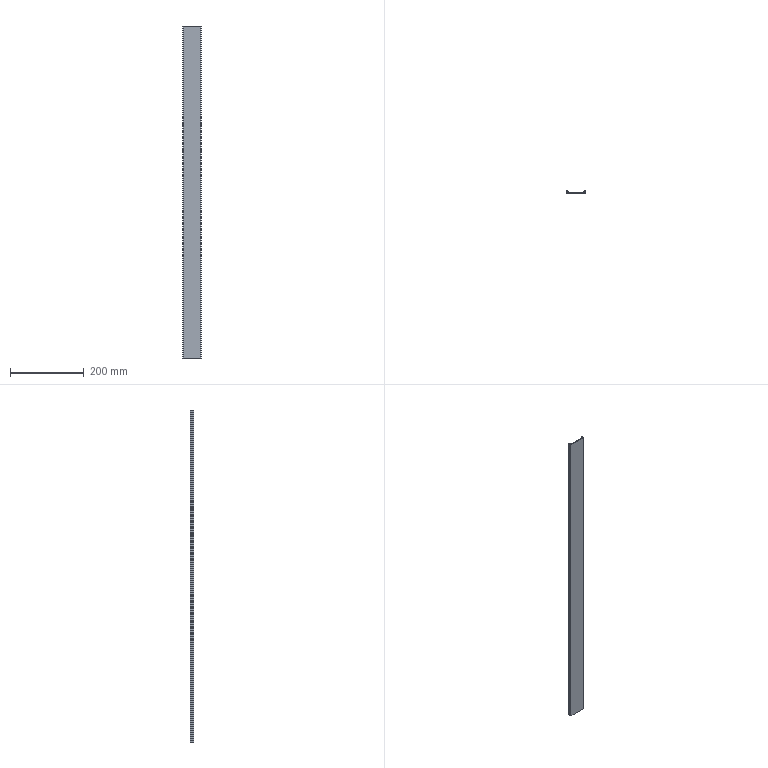Part | STEP file | 31E-01001CC13 | 1 solid | 32 faces | box 50 x 9.195 x 900 mm | volume 78943 mm3 | cylinder 16 | plane 16 | commonest cylinder face diameters 1 x8 1.2 x6 2 x2
STEP:
#1=CARTESIAN_POINT('',(0.2485,8.595,450.));
#2=VERTEX_POINT('',#1);
#3=CARTESIAN_POINT('',(0.4243,8.171,450.));
#4=VERTEX_POINT('',#3);
#5=CARTESIAN_POINT('',(0.8485,8.595,450.));
#6=DIRECTION('',(0.,0.,-1.));
#7=AXIS2_PLACEMENT_3D('',#5,#6,$);
#8=CIRCLE('',#7,0.6);
#9=EDGE_CURVE('',#2,#4,#8,.F.);
#10=ORIENTED_EDGE('',*,*,#9,.F.);
#11=CARTESIAN_POINT('',(0.2485,8.595,-450.));
#12=VERTEX_POINT('',#11);
#13=CARTESIAN_POINT('',(0.2485,8.595,450.));
#14=DIRECTION('',(0.,0.,-1.));
#15=VECTOR('',#14,1.);
#16=LINE('',#13,#15);
#17=EDGE_CURVE('',#2,#12,#16,.T.);
#18=ORIENTED_EDGE('',*,*,#17,.T.);
#19=CARTESIAN_POINT('',(0.4243,8.171,-450.));
#20=VERTEX_POINT('',#19);
#21=CARTESIAN_POINT('',(0.8485,8.595,-450.));
#22=DIRECTION('',(0.,0.,-1.));
#23=AXIS2_PLACEMENT_3D('',#21,#22,$);
#24=CIRCLE('',#23,0.6);
#25=EDGE_CURVE('',#20,#12,#24,.T.);
#26=ORIENTED_EDGE('',*,*,#25,.F.);
#27=CARTESIAN_POINT('',(0.4243,8.171,450.));
#28=DIRECTION('',(0.,0.,-1.));
#29=VECTOR('',#28,1.);
#30=LINE('',#27,#29);
#31=EDGE_CURVE('',#4,#20,#30,.T.);
#32=ORIENTED_EDGE('',*,*,#31,.F.);
#33=EDGE_LOOP('',(#10,#18,#26,#32));
#34=FACE_OUTER_BOUND('',#33,.T.);
#35=CARTESIAN_POINT('',(0.8485,8.595,450.));
#36=DIRECTION('',(0.,0.,-1.));
#37=DIRECTION('',(1.,0.,0.));
#38=AXIS2_PLACEMENT_3D('',#35,#36,#37);
#39=CYLINDRICAL_SURFACE('',#38,0.6);
#40=ADVANCED_FACE('',(#34),#39,.T.);
#41=CARTESIAN_POINT('',(1.273,9.019,450.));
#42=VERTEX_POINT('',#41);
#43=CARTESIAN_POINT('',(0.4243,9.019,450.));
#44=VERTEX_POINT('',#43);
#45=CARTESIAN_POINT('',(1.273,9.019,450.));
#46=CARTESIAN_POINT('',(1.219,9.073,450.));
#47=CARTESIAN_POINT('',(1.158,9.118,450.));
#48=CARTESIAN_POINT('',(1.089,9.152,450.));
#49=CARTESIAN_POINT('',(0.9442,9.199,450.));
#50=CARTESIAN_POINT('',(0.7916,9.2,450.));
#51=CARTESIAN_POINT('',(0.7159,9.188,450.));
#52=CARTESIAN_POINT('',(0.6071,9.152,450.));
#53=CARTESIAN_POINT('',(0.5104,9.093,450.));
#54=CARTESIAN_POINT('',(0.4796,9.07,450.));
#55=CARTESIAN_POINT('',(0.4509,9.046,450.));
#56=CARTESIAN_POINT('',(0.4243,9.019,450.));
#57=B_SPLINE_CURVE_WITH_KNOTS('',5,(#45,#46,#47,#48,#49,#50,#51,#52,#53,#54,#55,#56),.UNSPECIFIED.,.F.,.U.,(6,3,3,6),(0.,0.5331,1.066,1.332),.UNSPECIFIED.);
#58=EDGE_CURVE('',#42,#44,#57,.T.);
#59=ORIENTED_EDGE('',*,*,#58,.T.);
#60=CARTESIAN_POINT('',(0.4243,9.019,450.));
#61=CARTESIAN_POINT('',(0.3843,8.979,450.));
#62=CARTESIAN_POINT('',(0.349,8.935,450.));
#63=CARTESIAN_POINT('',(0.3192,8.886,450.));
#64=CARTESIAN_POINT('',(0.2795,8.8,450.));
#65=CARTESIAN_POINT('',(0.2574,8.708,450.));
#66=CARTESIAN_POINT('',(0.2515,8.67,450.));
#67=CARTESIAN_POINT('',(0.2485,8.633,450.));
#68=CARTESIAN_POINT('',(0.2485,8.595,450.));
#69=B_SPLINE_CURVE_WITH_KNOTS('',5,(#60,#61,#62,#63,#64,#65,#66,#67,#68),.UNSPECIFIED.,.F.,.U.,(6,3,6),(0.,0.3999,0.6659),.UNSPECIFIED.);
#70=EDGE_CURVE('',#44,#2,#69,.T.);
#71=ORIENTED_EDGE('',*,*,#70,.T.);
#72=ORIENTED_EDGE('',*,*,#9,.T.);
#73=CARTESIAN_POINT('',(2.898,5.697,450.));
#74=VERTEX_POINT('',#73);
#75=CARTESIAN_POINT('',(1.661,6.934,450.));
#76=DIRECTION('',(0.7071,-0.7071,0.));
#77=VECTOR('',#76,1.);
#78=LINE('',#75,#77);
#79=EDGE_CURVE('',#4,#74,#78,.T.);
#80=ORIENTED_EDGE('',*,*,#79,.T.);
#81=CARTESIAN_POINT('',(0.3706,5.02,450.));
#82=VERTEX_POINT('',#81);
#83=CARTESIAN_POINT('',(1.634,5.359,450.));
#84=DIRECTION('',(-0.9659,-0.2588,0.));
#85=VECTOR('',#84,1.);
#86=LINE('',#83,#85);
#87=EDGE_CURVE('',#74,#82,#86,.T.);
#88=ORIENTED_EDGE('',*,*,#87,.T.);
#89=CARTESIAN_POINT('',(0.,4.537,450.));
#90=VERTEX_POINT('',#89);
#91=CARTESIAN_POINT('',(0.3706,5.02,450.));
#92=CARTESIAN_POINT('',(0.32,5.007,450.));
#93=CARTESIAN_POINT('',(0.2712,4.986,450.));
#94=CARTESIAN_POINT('',(0.2253,4.96,450.));
#95=CARTESIAN_POINT('',(0.1416,4.896,450.));
#96=CARTESIAN_POINT('',(0.07725,4.812,450.));
#97=CARTESIAN_POINT('',(0.05076,4.766,450.));
#98=CARTESIAN_POINT('',(0.02052,4.693,450.));
#99=CARTESIAN_POINT('',(0.005155,4.616,450.));
#100=CARTESIAN_POINT('',(0.001709,4.589,450.));
#101=CARTESIAN_POINT('',(0.,4.563,450.));
#102=CARTESIAN_POINT('',(0.,4.537,450.));
#103=B_SPLINE_CURVE_WITH_KNOTS('',5,(#91,#92,#93,#94,#95,#96,#97,#98,#99,#100,#101,#102),.UNSPECIFIED.,.F.,.U.,(6,3,3,6),(0.,0.3702,0.7405,0.9253),.UNSPECIFIED.);
#104=EDGE_CURVE('',#82,#90,#103,.T.);
#105=ORIENTED_EDGE('',*,*,#104,.T.);
#106=CARTESIAN_POINT('',(0.,1.,450.));
#107=VERTEX_POINT('',#106);
#108=CARTESIAN_POINT('',(0.,2.769,450.));
#109=DIRECTION('',(0.,-1.,0.));
#110=VECTOR('',#109,1.);
#111=LINE('',#108,#110);
#112=EDGE_CURVE('',#90,#107,#111,.T.);
#113=ORIENTED_EDGE('',*,*,#112,.T.);
#114=CARTESIAN_POINT('',(1.,0.,450.));
#115=VERTEX_POINT('',#114);
#116=CARTESIAN_POINT('',(0.,1.,450.));
#117=CARTESIAN_POINT('',(0.,0.902,450.));
#118=CARTESIAN_POINT('',(0.012,0.804,450.));
#119=CARTESIAN_POINT('',(0.036,0.708,450.));
#120=CARTESIAN_POINT('',(0.107,0.5238,450.));
#121=CARTESIAN_POINT('',(0.2204,0.3622,450.));
#122=CARTESIAN_POINT('',(0.2868,0.2888,450.));
#123=CARTESIAN_POINT('',(0.4361,0.1597,450.));
#124=CARTESIAN_POINT('',(0.6122,0.0704,450.));
#125=CARTESIAN_POINT('',(0.7053,0.03682,450.));
#126=CARTESIAN_POINT('',(0.8215,0.01049,450.));
#127=CARTESIAN_POINT('',(0.9393,0.001534,450.));
#128=CARTESIAN_POINT('',(0.9596,0.0005109,450.));
#129=CARTESIAN_POINT('',(0.9798,0.000000001,450.));
#130=CARTESIAN_POINT('',(1.,0.000000001,450.));
#131=B_SPLINE_CURVE_WITH_KNOTS('',5,(#116,#117,#118,#119,#120,#121,#122,#123,#124,#125,#126,#127,#128,#129,#130),.UNSPECIFIED.,.F.,.U.,(6,3,3,3,6),(0.,0.6928,1.386,2.078,2.221),.UNSPECIFIED.);
#132=EDGE_CURVE('',#107,#115,#131,.T.);
#133=ORIENTED_EDGE('',*,*,#132,.T.);
#134=CARTESIAN_POINT('',(49.,0.,450.));
#135=VERTEX_POINT('',#134);
#136=CARTESIAN_POINT('',(25.,0.000000001,450.));
#137=DIRECTION('',(1.,0.,0.));
#138=VECTOR('',#137,1.);
#139=LINE('',#136,#138);
#140=EDGE_CURVE('',#115,#135,#139,.T.);
#141=ORIENTED_EDGE('',*,*,#140,.T.);
#142=CARTESIAN_POINT('',(50.,1.,450.));
#143=VERTEX_POINT('',#142);
#144=CARTESIAN_POINT('',(49.,0.000000001,450.));
#145=CARTESIAN_POINT('',(49.098,0.000000001,450.));
#146=CARTESIAN_POINT('',(49.196,0.012,450.));
#147=CARTESIAN_POINT('',(49.292,0.036,450.));
#148=CARTESIAN_POINT('',(49.476,0.107,450.));
#149=CARTESIAN_POINT('',(49.638,0.2204,450.));
#150=CARTESIAN_POINT('',(49.711,0.2868,450.));
#151=CARTESIAN_POINT('',(49.84,0.4361,450.));
#152=CARTESIAN_POINT('',(49.93,0.6122,450.));
#153=CARTESIAN_POINT('',(49.963,0.7053,450.));
#154=CARTESIAN_POINT('',(49.99,0.8215,450.));
#155=CARTESIAN_POINT('',(49.998,0.9393,450.));
#156=CARTESIAN_POINT('',(49.999,0.9596,450.));
#157=CARTESIAN_POINT('',(50.,0.9798,450.));
#158=CARTESIAN_POINT('',(50.,1.,450.));
#159=B_SPLINE_CURVE_WITH_KNOTS('',5,(#144,#145,#146,#147,#148,#149,#150,#151,#152,#153,#154,#155,#156,#157,#158),.UNSPECIFIED.,.F.,.U.,(6,3,3,3,6),(0.,0.6928,1.386,2.078,2.221),.UNSPECIFIED.);
#160=EDGE_CURVE('',#135,#143,#159,.T.);
#161=ORIENTED_EDGE('',*,*,#160,.T.);
#162=CARTESIAN_POINT('',(50.,4.537,450.));
#163=VERTEX_POINT('',#162);
#164=CARTESIAN_POINT('',(50.,2.769,450.));
#165=DIRECTION('',(0.,1.,0.));
#166=VECTOR('',#165,1.);
#167=LINE('',#164,#166);
#168=EDGE_CURVE('',#143,#163,#167,.T.);
#169=ORIENTED_EDGE('',*,*,#168,.T.);
#170=CARTESIAN_POINT('',(49.629,5.02,450.));
#171=VERTEX_POINT('',#170);
#172=CARTESIAN_POINT('',(50.,4.537,450.));
#173=CARTESIAN_POINT('',(50.,4.589,450.));
#174=CARTESIAN_POINT('',(49.993,4.642,450.));
#175=CARTESIAN_POINT('',(49.979,4.693,450.));
#176=CARTESIAN_POINT('',(49.939,4.791,450.));
#177=CARTESIAN_POINT('',(49.875,4.874,450.));
#178=CARTESIAN_POINT('',(49.837,4.912,450.));
#179=CARTESIAN_POINT('',(49.774,4.96,450.));
#180=CARTESIAN_POINT('',(49.704,4.995,450.));
#181=CARTESIAN_POINT('',(49.679,5.005,450.));
#182=CARTESIAN_POINT('',(49.655,5.013,450.));
#183=CARTESIAN_POINT('',(49.629,5.02,450.));
#184=B_SPLINE_CURVE_WITH_KNOTS('',5,(#172,#173,#174,#175,#176,#177,#178,#179,#180,#181,#182,#183),.UNSPECIFIED.,.F.,.U.,(6,3,3,6),(0.,0.3702,0.7405,0.9253),.UNSPECIFIED.);
#185=EDGE_CURVE('',#163,#171,#184,.T.);
#186=ORIENTED_EDGE('',*,*,#185,.T.);
#187=CARTESIAN_POINT('',(47.102,5.697,450.));
#188=VERTEX_POINT('',#187);
#189=CARTESIAN_POINT('',(48.366,5.359,450.));
#190=DIRECTION('',(-0.9659,0.2588,0.));
#191=VECTOR('',#190,1.);
#192=LINE('',#189,#191);
#193=EDGE_CURVE('',#171,#188,#192,.T.);
#194=ORIENTED_EDGE('',*,*,#193,.T.);
#195=CARTESIAN_POINT('',(49.576,8.171,450.));
#196=VERTEX_POINT('',#195);
#197=CARTESIAN_POINT('',(48.339,6.934,450.));
#198=DIRECTION('',(0.7071,0.7071,0.));
#199=VECTOR('',#198,1.);
#200=LINE('',#197,#199);
#201=EDGE_CURVE('',#188,#196,#200,.T.);
#202=ORIENTED_EDGE('',*,*,#201,.T.);
#203=CARTESIAN_POINT('',(49.751,8.595,450.));
#204=VERTEX_POINT('',#203);
#205=CARTESIAN_POINT('',(49.576,8.171,450.));
#206=CARTESIAN_POINT('',(49.629,8.224,450.));
#207=CARTESIAN_POINT('',(49.674,8.286,450.));
#208=CARTESIAN_POINT('',(49.709,8.354,450.));
#209=CARTESIAN_POINT('',(49.738,8.445,450.));
#210=CARTESIAN_POINT('',(49.749,8.539,450.));
#211=CARTESIAN_POINT('',(49.751,8.557,450.));
#212=CARTESIAN_POINT('',(49.751,8.576,450.));
#213=CARTESIAN_POINT('',(49.751,8.595,450.));
#214=B_SPLINE_CURVE_WITH_KNOTS('',5,(#205,#206,#207,#208,#209,#210,#211,#212,#213),.UNSPECIFIED.,.F.,.U.,(6,3,6),(0.,0.5331,0.6664),.UNSPECIFIED.);
#215=EDGE_CURVE('',#196,#204,#214,.T.);
#216=ORIENTED_EDGE('',*,*,#215,.T.);
#217=CARTESIAN_POINT('',(49.576,9.019,450.));
#218=VERTEX_POINT('',#217);
#219=CARTESIAN_POINT('',(49.751,8.595,450.));
#220=CARTESIAN_POINT('',(49.751,8.652,450.));
#221=CARTESIAN_POINT('',(49.745,8.708,450.));
#222=CARTESIAN_POINT('',(49.731,8.764,450.));
#223=CARTESIAN_POINT('',(49.699,8.853,450.));
#224=CARTESIAN_POINT('',(49.649,8.933,450.));
#225=CARTESIAN_POINT('',(49.627,8.964,450.));
#226=CARTESIAN_POINT('',(49.602,8.993,450.));
#227=CARTESIAN_POINT('',(49.576,9.019,450.));
#228=B_SPLINE_CURVE_WITH_KNOTS('',5,(#219,#220,#221,#222,#223,#224,#225,#226,#227),.UNSPECIFIED.,.F.,.U.,(6,3,6),(0.6664,1.066,1.332),.UNSPECIFIED.);
#229=EDGE_CURVE('',#204,#218,#228,.T.);
#230=ORIENTED_EDGE('',*,*,#229,.T.);
#231=CARTESIAN_POINT('',(48.727,9.019,450.));
#232=VERTEX_POINT('',#231);
#233=CARTESIAN_POINT('',(49.576,9.019,450.));
#234=CARTESIAN_POINT('',(49.522,9.073,450.));
#235=CARTESIAN_POINT('',(49.461,9.118,450.));
#236=CARTESIAN_POINT('',(49.392,9.152,450.));
#237=CARTESIAN_POINT('',(49.247,9.199,450.));
#238=CARTESIAN_POINT('',(49.095,9.2,450.));
#239=CARTESIAN_POINT('',(49.019,9.188,450.));
#240=CARTESIAN_POINT('',(48.91,9.152,450.));
#241=CARTESIAN_POINT('',(48.813,9.093,450.));
#242=CARTESIAN_POINT('',(48.782,9.07,450.));
#243=CARTESIAN_POINT('',(48.754,9.046,450.));
#244=CARTESIAN_POINT('',(48.727,9.019,450.));
#245=B_SPLINE_CURVE_WITH_KNOTS('',5,(#233,#234,#235,#236,#237,#238,#239,#240,#241,#242,#243,#244),.UNSPECIFIED.,.F.,.U.,(6,3,3,6),(0.,0.5331,1.066,1.332),.UNSPECIFIED.);
#246=EDGE_CURVE('',#218,#232,#245,.T.);
#247=ORIENTED_EDGE('',*,*,#246,.T.);
#248=CARTESIAN_POINT('',(45.396,5.688,450.));
#249=VERTEX_POINT('',#248);
#250=CARTESIAN_POINT('',(47.062,7.354,450.));
#251=DIRECTION('',(-0.7071,-0.7071,0.));
#252=VECTOR('',#251,1.);
#253=LINE('',#250,#252);
#254=EDGE_CURVE('',#232,#249,#253,.T.);
#255=ORIENTED_EDGE('',*,*,#254,.T.);
#256=CARTESIAN_POINT('',(45.25,5.335,450.));
#257=VERTEX_POINT('',#256);
#258=CARTESIAN_POINT('',(45.396,5.688,450.));
#259=CARTESIAN_POINT('',(45.363,5.655,450.));
#260=CARTESIAN_POINT('',(45.334,5.618,450.));
#261=CARTESIAN_POINT('',(45.309,5.577,450.));
#262=CARTESIAN_POINT('',(45.276,5.506,450.));
#263=CARTESIAN_POINT('',(45.257,5.429,450.));
#264=CARTESIAN_POINT('',(45.252,5.398,450.));
#265=CARTESIAN_POINT('',(45.25,5.366,450.));
#266=CARTESIAN_POINT('',(45.25,5.335,450.));
#267=B_SPLINE_CURVE_WITH_KNOTS('',5,(#258,#259,#260,#261,#262,#263,#264,#265,#266),.UNSPECIFIED.,.F.,.U.,(6,3,6),(0.,0.3332,0.5549),.UNSPECIFIED.);
#268=EDGE_CURVE('',#249,#257,#267,.T.);
#269=ORIENTED_EDGE('',*,*,#268,.T.);
#270=CARTESIAN_POINT('',(45.621,4.852,450.));
#271=VERTEX_POINT('',#270);
#272=CARTESIAN_POINT('',(45.25,5.335,450.));
#273=CARTESIAN_POINT('',(45.25,5.283,450.));
#274=CARTESIAN_POINT('',(45.257,5.23,450.));
#275=CARTESIAN_POINT('',(45.27,5.179,450.));
#276=CARTESIAN_POINT('',(45.311,5.081,450.));
#277=CARTESIAN_POINT('',(45.375,4.998,450.));
#278=CARTESIAN_POINT('',(45.413,4.96,450.));
#279=CARTESIAN_POINT('',(45.476,4.912,450.));
#280=CARTESIAN_POINT('',(45.546,4.877,450.));
#281=CARTESIAN_POINT('',(45.57,4.867,450.));
#282=CARTESIAN_POINT('',(45.595,4.859,450.));
#283=CARTESIAN_POINT('',(45.621,4.852,450.));
#284=B_SPLINE_CURVE_WITH_KNOTS('',5,(#272,#273,#274,#275,#276,#277,#278,#279,#280,#281,#282,#283),.UNSPECIFIED.,.F.,.U.,(6,3,3,6),(0.,0.3702,0.7405,0.9253),.UNSPECIFIED.);
#285=EDGE_CURVE('',#257,#271,#284,.T.);
#286=ORIENTED_EDGE('',*,*,#285,.T.);
#287=CARTESIAN_POINT('',(48.8,4.,450.));
#288=VERTEX_POINT('',#287);
#289=CARTESIAN_POINT('',(47.21,4.426,450.));
#290=DIRECTION('',(0.9659,-0.2588,0.));
#291=VECTOR('',#290,1.);
#292=LINE('',#289,#291);
#293=EDGE_CURVE('',#271,#288,#292,.T.);
#294=ORIENTED_EDGE('',*,*,#293,.T.);
#295=CARTESIAN_POINT('',(48.8,1.7,450.));
#296=VERTEX_POINT('',#295);
#297=CARTESIAN_POINT('',(48.8,2.85,450.));
#298=DIRECTION('',(0.,-1.,0.));
#299=VECTOR('',#298,1.);
#300=LINE('',#297,#299);
#301=EDGE_CURVE('',#288,#296,#300,.T.);
#302=ORIENTED_EDGE('',*,*,#301,.T.);
#303=CARTESIAN_POINT('',(48.3,1.2,450.));
#304=VERTEX_POINT('',#303);
#305=CARTESIAN_POINT('',(48.3,1.7,450.));
#306=DIRECTION('',(0.,0.,-1.));
#307=AXIS2_PLACEMENT_3D('',#305,#306,$);
#308=CIRCLE('',#307,0.5);
#309=EDGE_CURVE('',#296,#304,#308,.T.);
#310=ORIENTED_EDGE('',*,*,#309,.T.);
#311=CARTESIAN_POINT('',(1.7,1.2,450.));
#312=VERTEX_POINT('',#311);
#313=CARTESIAN_POINT('',(25.,1.2,450.));
#314=DIRECTION('',(-1.,0.,0.));
#315=VECTOR('',#314,1.);
#316=LINE('',#313,#315);
#317=EDGE_CURVE('',#304,#312,#316,.T.);
#318=ORIENTED_EDGE('',*,*,#317,.T.);
#319=CARTESIAN_POINT('',(1.2,1.7,450.));
#320=VERTEX_POINT('',#319);
#321=CARTESIAN_POINT('',(1.7,1.7,450.));
#322=DIRECTION('',(0.,0.,-1.));
#323=AXIS2_PLACEMENT_3D('',#321,#322,$);
#324=CIRCLE('',#323,0.5);
#325=EDGE_CURVE('',#312,#320,#324,.T.);
#326=ORIENTED_EDGE('',*,*,#325,.T.);
#327=CARTESIAN_POINT('',(1.2,4.,450.));
#328=VERTEX_POINT('',#327);
#329=CARTESIAN_POINT('',(1.2,2.85,450.));
#330=DIRECTION('',(0.,1.,0.));
#331=VECTOR('',#330,1.);
#332=LINE('',#329,#331);
#333=EDGE_CURVE('',#320,#328,#332,.T.);
#334=ORIENTED_EDGE('',*,*,#333,.T.);
#335=CARTESIAN_POINT('',(4.379,4.852,450.));
#336=VERTEX_POINT('',#335);
#337=CARTESIAN_POINT('',(2.79,4.426,450.));
#338=DIRECTION('',(0.9659,0.2588,0.));
#339=VECTOR('',#338,1.);
#340=LINE('',#337,#339);
#341=EDGE_CURVE('',#328,#336,#340,.T.);
#342=ORIENTED_EDGE('',*,*,#341,.T.);
#343=CARTESIAN_POINT('',(4.75,5.335,450.));
#344=VERTEX_POINT('',#343);
#345=CARTESIAN_POINT('',(4.379,4.852,450.));
#346=CARTESIAN_POINT('',(4.446,4.87,450.));
#347=CARTESIAN_POINT('',(4.51,4.899,450.));
#348=CARTESIAN_POINT('',(4.568,4.94,450.));
#349=CARTESIAN_POINT('',(4.662,5.034,450.));
#350=CARTESIAN_POINT('',(4.722,5.152,450.));
#351=CARTESIAN_POINT('',(4.741,5.212,450.));
#352=CARTESIAN_POINT('',(4.75,5.273,450.));
#353=CARTESIAN_POINT('',(4.75,5.335,450.));
#354=B_SPLINE_CURVE_WITH_KNOTS('',5,(#345,#346,#347,#348,#349,#350,#351,#352,#353),.UNSPECIFIED.,.F.,.U.,(6,3,6),(0.,0.4899,0.9256),.UNSPECIFIED.);
#355=EDGE_CURVE('',#336,#344,#354,.T.);
#356=ORIENTED_EDGE('',*,*,#355,.T.);
#357=CARTESIAN_POINT('',(4.604,5.688,450.));
#358=VERTEX_POINT('',#357);
#359=CARTESIAN_POINT('',(4.75,5.335,450.));
#360=CARTESIAN_POINT('',(4.75,5.343,450.));
#361=CARTESIAN_POINT('',(4.75,5.35,450.));
#362=CARTESIAN_POINT('',(4.75,5.358,450.));
#363=CARTESIAN_POINT('',(4.745,5.435,450.));
#364=CARTESIAN_POINT('',(4.726,5.51,450.));
#365=CARTESIAN_POINT('',(4.697,5.575,450.));
#366=CARTESIAN_POINT('',(4.657,5.634,450.));
#367=CARTESIAN_POINT('',(4.607,5.685,450.));
#368=CARTESIAN_POINT('',(4.606,5.686,450.));
#369=CARTESIAN_POINT('',(4.605,5.687,450.));
#370=CARTESIAN_POINT('',(4.604,5.688,450.));
#371=B_SPLINE_CURVE_WITH_KNOTS('',5,(#359,#360,#361,#362,#363,#364,#365,#366,#367,#368,#369,#370),.UNSPECIFIED.,.F.,.U.,(6,3,3,6),(0.9256,0.9798,1.47,1.481),.UNSPECIFIED.);
#372=EDGE_CURVE('',#344,#358,#371,.T.);
#373=ORIENTED_EDGE('',*,*,#372,.T.);
#374=CARTESIAN_POINT('',(2.938,7.354,450.));
#375=DIRECTION('',(-0.7071,0.7071,0.));
#376=VECTOR('',#375,1.);
#377=LINE('',#374,#376);
#378=EDGE_CURVE('',#358,#42,#377,.T.);
#379=ORIENTED_EDGE('',*,*,#378,.T.);
#380=EDGE_LOOP('',(#59,#71,#72,#80,#88,#105,#113,#133,#141,#161,#169,#186,#194,#202,#216,#230,#247,#255,#269,#286,#294,#302,#310,#318,#326,#334,#342,#356,#373,#379));
#381=FACE_OUTER_BOUND('',#380,.T.);
#382=CARTESIAN_POINT('',(0.,1.2,450.));
#383=DIRECTION('',(0.,0.,-1.));
#384=DIRECTION('',(-1.,0.,0.));
#385=AXIS2_PLACEMENT_3D('',#382,#383,#384);
#386=PLANE('',#385);
#387=ADVANCED_FACE('',(#381),#386,.F.);
#388=ORIENTED_EDGE('',*,*,#17,.F.);
#389=ORIENTED_EDGE('',*,*,#70,.F.);
#390=CARTESIAN_POINT('',(0.4243,9.019,-450.));
#391=VERTEX_POINT('',#390);
#392=CARTESIAN_POINT('',(0.4243,9.019,450.));
#393=DIRECTION('',(0.,0.,-1.));
#394=VECTOR('',#393,1.);
#395=LINE('',#392,#394);
#396=EDGE_CURVE('',#44,#391,#395,.T.);
#397=ORIENTED_EDGE('',*,*,#396,.T.);
#398=CARTESIAN_POINT('',(0.8485,8.595,-450.));
#399=DIRECTION('',(0.,0.,-1.));
#400=AXIS2_PLACEMENT_3D('',#398,#399,$);
#401=CIRCLE('',#400,0.6);
#402=EDGE_CURVE('',#12,#391,#401,.T.);
#403=ORIENTED_EDGE('',*,*,#402,.F.);
#404=EDGE_LOOP('',(#388,#389,#397,#403));
#405=FACE_OUTER_BOUND('',#404,.T.);
#406=CARTESIAN_POINT('',(0.8485,8.595,450.));
#407=DIRECTION('',(0.,0.,-1.));
#408=DIRECTION('',(-1.,0.,0.));
#409=AXIS2_PLACEMENT_3D('',#406,#407,#408);
#410=CYLINDRICAL_SURFACE('',#409,0.6);
#411=ADVANCED_FACE('',(#405),#410,.T.);
#412=CARTESIAN_POINT('',(2.898,5.697,-450.));
#413=VERTEX_POINT('',#412);
#414=CARTESIAN_POINT('',(1.661,6.934,-450.));
#415=DIRECTION('',(0.7071,-0.7071,0.));
#416=VECTOR('',#415,1.);
#417=LINE('',#414,#416);
#418=EDGE_CURVE('',#20,#413,#417,.T.);
#419=ORIENTED_EDGE('',*,*,#418,.F.);
#420=ORIENTED_EDGE('',*,*,#25,.T.);
#421=ORIENTED_EDGE('',*,*,#402,.T.);
#422=CARTESIAN_POINT('',(1.273,9.019,-450.));
#423=VERTEX_POINT('',#422);
#424=CARTESIAN_POINT('',(0.8485,8.595,-450.));
#425=DIRECTION('',(0.,0.,-1.));
#426=AXIS2_PLACEMENT_3D('',#424,#425,$);
#427=CIRCLE('',#426,0.6);
#428=EDGE_CURVE('',#391,#423,#427,.T.);
#429=ORIENTED_EDGE('',*,*,#428,.T.);
#430=CARTESIAN_POINT('',(4.604,5.688,-450.));
#431=VERTEX_POINT('',#430);
#432=CARTESIAN_POINT('',(2.938,7.354,-450.));
#433=DIRECTION('',(-0.7071,0.7071,0.));
#434=VECTOR('',#433,1.);
#435=LINE('',#432,#434);
#436=EDGE_CURVE('',#431,#423,#435,.T.);
#437=ORIENTED_EDGE('',*,*,#436,.F.);
#438=CARTESIAN_POINT('',(4.75,5.335,-450.));
#439=VERTEX_POINT('',#438);
#440=CARTESIAN_POINT('',(4.25,5.335,-450.));
#441=DIRECTION('',(0.,0.,-1.));
#442=AXIS2_PLACEMENT_3D('',#440,#441,$);
#443=CIRCLE('',#442,0.5);
#444=EDGE_CURVE('',#431,#439,#443,.T.);
#445=ORIENTED_EDGE('',*,*,#444,.T.);
#446=CARTESIAN_POINT('',(4.379,4.852,-450.));
#447=VERTEX_POINT('',#446);
#448=CARTESIAN_POINT('',(4.25,5.335,-450.));
#449=DIRECTION('',(0.,0.,-1.));
#450=AXIS2_PLACEMENT_3D('',#448,#449,$);
#451=CIRCLE('',#450,0.5);
#452=EDGE_CURVE('',#439,#447,#451,.T.);
#453=ORIENTED_EDGE('',*,*,#452,.T.);
#454=CARTESIAN_POINT('',(1.2,4.,-450.));
#455=VERTEX_POINT('',#454);
#456=CARTESIAN_POINT('',(2.79,4.426,-450.));
#457=DIRECTION('',(0.9659,0.2588,0.));
#458=VECTOR('',#457,1.);
#459=LINE('',#456,#458);
#460=EDGE_CURVE('',#455,#447,#459,.T.);
#461=ORIENTED_EDGE('',*,*,#460,.F.);
#462=CARTESIAN_POINT('',(1.2,1.7,-450.));
#463=VERTEX_POINT('',#462);
#464=CARTESIAN_POINT('',(1.2,2.85,-450.));
#465=DIRECTION('',(0.,1.,0.));
#466=VECTOR('',#465,1.);
#467=LINE('',#464,#466);
#468=EDGE_CURVE('',#463,#455,#467,.T.);
#469=ORIENTED_EDGE('',*,*,#468,.F.);
#470=CARTESIAN_POINT('',(1.7,1.2,-450.));
#471=VERTEX_POINT('',#470);
#472=CARTESIAN_POINT('',(1.2,1.7,-450.));
#473=CARTESIAN_POINT('',(1.2,1.637,-450.));
#474=CARTESIAN_POINT('',(1.21,1.574,-450.));
#475=CARTESIAN_POINT('',(1.23,1.514,-450.));
#476=CARTESIAN_POINT('',(1.288,1.4,-450.));
#477=CARTESIAN_POINT('',(1.377,1.31,-450.));
#478=CARTESIAN_POINT('',(1.429,1.273,-450.));
#479=CARTESIAN_POINT('',(1.514,1.23,-450.));
#480=CARTESIAN_POINT('',(1.606,1.207,-450.));
#481=CARTESIAN_POINT('',(1.637,1.202,-450.));
#482=CARTESIAN_POINT('',(1.669,1.2,-450.));
#483=CARTESIAN_POINT('',(1.7,1.2,-450.));
#484=B_SPLINE_CURVE_WITH_KNOTS('',5,(#472,#473,#474,#475,#476,#477,#478,#479,#480,#481,#482,#483),.UNSPECIFIED.,.F.,.U.,(6,3,3,6),(0.,0.4443,0.8886,1.11),.UNSPECIFIED.);
#485=EDGE_CURVE('',#463,#471,#484,.T.);
#486=ORIENTED_EDGE('',*,*,#485,.T.);
#487=CARTESIAN_POINT('',(48.3,1.2,-450.));
#488=VERTEX_POINT('',#487);
#489=CARTESIAN_POINT('',(25.,1.2,-450.));
#490=DIRECTION('',(-1.,0.,0.));
#491=VECTOR('',#490,1.);
#492=LINE('',#489,#491);
#493=EDGE_CURVE('',#488,#471,#492,.T.);
#494=ORIENTED_EDGE('',*,*,#493,.F.);
#495=CARTESIAN_POINT('',(48.8,1.7,-450.));
#496=VERTEX_POINT('',#495);
#497=CARTESIAN_POINT('',(48.3,1.2,-450.));
#498=CARTESIAN_POINT('',(48.363,1.2,-450.));
#499=CARTESIAN_POINT('',(48.426,1.21,-450.));
#500=CARTESIAN_POINT('',(48.486,1.23,-450.));
#501=CARTESIAN_POINT('',(48.6,1.288,-450.));
#502=CARTESIAN_POINT('',(48.69,1.377,-450.));
#503=CARTESIAN_POINT('',(48.727,1.429,-450.));
#504=CARTESIAN_POINT('',(48.77,1.514,-450.));
#505=CARTESIAN_POINT('',(48.793,1.606,-450.));
#506=CARTESIAN_POINT('',(48.798,1.637,-450.));
#507=CARTESIAN_POINT('',(48.8,1.669,-450.));
#508=CARTESIAN_POINT('',(48.8,1.7,-450.));
#509=B_SPLINE_CURVE_WITH_KNOTS('',5,(#497,#498,#499,#500,#501,#502,#503,#504,#505,#506,#507,#508),.UNSPECIFIED.,.F.,.U.,(6,3,3,6),(0.,0.4443,0.8886,1.11),.UNSPECIFIED.);
#510=EDGE_CURVE('',#488,#496,#509,.T.);
#511=ORIENTED_EDGE('',*,*,#510,.T.);
#512=CARTESIAN_POINT('',(48.8,4.,-450.));
#513=VERTEX_POINT('',#512);
#514=CARTESIAN_POINT('',(48.8,2.85,-450.));
#515=DIRECTION('',(0.,-1.,0.));
#516=VECTOR('',#515,1.);
#517=LINE('',#514,#516);
#518=EDGE_CURVE('',#513,#496,#517,.T.);
#519=ORIENTED_EDGE('',*,*,#518,.F.);
#520=CARTESIAN_POINT('',(45.621,4.852,-450.));
#521=VERTEX_POINT('',#520);
#522=CARTESIAN_POINT('',(47.21,4.426,-450.));
#523=DIRECTION('',(0.9659,-0.2588,0.));
#524=VECTOR('',#523,1.);
#525=LINE('',#522,#524);
#526=EDGE_CURVE('',#521,#513,#525,.T.);
#527=ORIENTED_EDGE('',*,*,#526,.F.);
#528=CARTESIAN_POINT('',(45.25,5.335,-450.));
#529=VERTEX_POINT('',#528);
#530=CARTESIAN_POINT('',(45.75,5.335,-450.));
#531=DIRECTION('',(0.,0.,-1.));
#532=AXIS2_PLACEMENT_3D('',#530,#531,$);
#533=CIRCLE('',#532,0.5);
#534=EDGE_CURVE('',#521,#529,#533,.T.);
#535=ORIENTED_EDGE('',*,*,#534,.T.);
#536=CARTESIAN_POINT('',(45.396,5.688,-450.));
#537=VERTEX_POINT('',#536);
#538=CARTESIAN_POINT('',(45.75,5.335,-450.));
#539=DIRECTION('',(0.,0.,-1.));
#540=AXIS2_PLACEMENT_3D('',#538,#539,$);
#541=CIRCLE('',#540,0.5);
#542=EDGE_CURVE('',#529,#537,#541,.T.);
#543=ORIENTED_EDGE('',*,*,#542,.T.);
#544=CARTESIAN_POINT('',(48.727,9.019,-450.));
#545=VERTEX_POINT('',#544);
#546=CARTESIAN_POINT('',(47.062,7.354,-450.));
#547=DIRECTION('',(-0.7071,-0.7071,0.));
#548=VECTOR('',#547,1.);
#549=LINE('',#546,#548);
#550=EDGE_CURVE('',#545,#537,#549,.T.);
#551=ORIENTED_EDGE('',*,*,#550,.F.);
#552=CARTESIAN_POINT('',(49.576,9.019,-450.));
#553=VERTEX_POINT('',#552);
#554=CARTESIAN_POINT('',(49.151,8.595,-450.));
#555=DIRECTION('',(0.,0.,-1.));
#556=AXIS2_PLACEMENT_3D('',#554,#555,$);
#557=CIRCLE('',#556,0.6);
#558=EDGE_CURVE('',#545,#553,#557,.T.);
#559=ORIENTED_EDGE('',*,*,#558,.T.);
#560=CARTESIAN_POINT('',(49.751,8.595,-450.));
#561=VERTEX_POINT('',#560);
#562=CARTESIAN_POINT('',(49.151,8.595,-450.));
#563=DIRECTION('',(0.,0.,-1.));
#564=AXIS2_PLACEMENT_3D('',#562,#563,$);
#565=CIRCLE('',#564,0.6);
#566=EDGE_CURVE('',#553,#561,#565,.T.);
#567=ORIENTED_EDGE('',*,*,#566,.T.);
#568=CARTESIAN_POINT('',(49.576,8.171,-450.));
#569=VERTEX_POINT('',#568);
#570=CARTESIAN_POINT('',(49.151,8.595,-450.));
#571=DIRECTION('',(0.,0.,-1.));
#572=AXIS2_PLACEMENT_3D('',#570,#571,$);
#573=CIRCLE('',#572,0.6);
#574=EDGE_CURVE('',#561,#569,#573,.T.);
#575=ORIENTED_EDGE('',*,*,#574,.T.);
#576=CARTESIAN_POINT('',(47.102,5.697,-450.));
#577=VERTEX_POINT('',#576);
#578=CARTESIAN_POINT('',(48.339,6.934,-450.));
#579=DIRECTION('',(0.7071,0.7071,0.));
#580=VECTOR('',#579,1.);
#581=LINE('',#578,#580);
#582=EDGE_CURVE('',#577,#569,#581,.T.);
#583=ORIENTED_EDGE('',*,*,#582,.F.);
#584=CARTESIAN_POINT('',(49.629,5.02,-450.));
#585=VERTEX_POINT('',#584);
#586=CARTESIAN_POINT('',(48.366,5.359,-450.));
#587=DIRECTION('',(-0.9659,0.2588,0.));
#588=VECTOR('',#587,1.);
#589=LINE('',#586,#588);
#590=EDGE_CURVE('',#585,#577,#589,.T.);
#591=ORIENTED_EDGE('',*,*,#590,.F.);
#592=CARTESIAN_POINT('',(50.,4.537,-450.));
#593=VERTEX_POINT('',#592);
#594=CARTESIAN_POINT('',(49.5,4.537,-450.));
#595=DIRECTION('',(0.,0.,-1.));
#596=AXIS2_PLACEMENT_3D('',#594,#595,$);
#597=CIRCLE('',#596,0.5);
#598=EDGE_CURVE('',#585,#593,#597,.T.);
#599=ORIENTED_EDGE('',*,*,#598,.T.);
#600=CARTESIAN_POINT('',(50.,1.,-450.));
#601=VERTEX_POINT('',#600);
#602=CARTESIAN_POINT('',(50.,2.769,-450.));
#603=DIRECTION('',(0.,1.,0.));
#604=VECTOR('',#603,1.);
#605=LINE('',#602,#604);
#606=EDGE_CURVE('',#601,#593,#605,.T.);
#607=ORIENTED_EDGE('',*,*,#606,.F.);
#608=CARTESIAN_POINT('',(49.,0.,-450.));
#609=VERTEX_POINT('',#608);
#610=CARTESIAN_POINT('',(49.,1.,-450.));
#611=DIRECTION('',(0.,0.,-1.));
#612=AXIS2_PLACEMENT_3D('',#610,#611,$);
#613=CIRCLE('',#612,1.);
#614=EDGE_CURVE('',#601,#609,#613,.T.);
#615=ORIENTED_EDGE('',*,*,#614,.T.);
#616=CARTESIAN_POINT('',(1.,0.,-450.));
#617=VERTEX_POINT('',#616);
#618=CARTESIAN_POINT('',(25.,0.000000001,-450.));
#619=DIRECTION('',(1.,0.,0.));
#620=VECTOR('',#619,1.);
#621=LINE('',#618,#620);
#622=EDGE_CURVE('',#617,#609,#621,.T.);
#623=ORIENTED_EDGE('',*,*,#622,.F.);
#624=CARTESIAN_POINT('',(0.,1.,-450.));
#625=VERTEX_POINT('',#624);
#626=CARTESIAN_POINT('',(1.,1.,-450.));
#627=DIRECTION('',(0.,0.,-1.));
#628=AXIS2_PLACEMENT_3D('',#626,#627,$);
#629=CIRCLE('',#628,1.);
#630=EDGE_CURVE('',#617,#625,#629,.T.);
#631=ORIENTED_EDGE('',*,*,#630,.T.);
#632=CARTESIAN_POINT('',(0.,4.537,-450.));
#633=VERTEX_POINT('',#632);
#634=CARTESIAN_POINT('',(0.,2.769,-450.));
#635=DIRECTION('',(0.,-1.,0.));
#636=VECTOR('',#635,1.);
#637=LINE('',#634,#636);
#638=EDGE_CURVE('',#633,#625,#637,.T.);
#639=ORIENTED_EDGE('',*,*,#638,.F.);
#640=CARTESIAN_POINT('',(0.3706,5.02,-450.));
#641=VERTEX_POINT('',#640);
#642=CARTESIAN_POINT('',(0.5,4.537,-450.));
#643=DIRECTION('',(0.,0.,-1.));
#644=AXIS2_PLACEMENT_3D('',#642,#643,$);
#645=CIRCLE('',#644,0.5);
#646=EDGE_CURVE('',#633,#641,#645,.T.);
#647=ORIENTED_EDGE('',*,*,#646,.T.);
#648=CARTESIAN_POINT('',(1.634,5.359,-450.));
#649=DIRECTION('',(-0.9659,-0.2588,0.));
#650=VECTOR('',#649,1.);
#651=LINE('',#648,#650);
#652=EDGE_CURVE('',#413,#641,#651,.T.);
#653=ORIENTED_EDGE('',*,*,#652,.F.);
#654=EDGE_LOOP('',(#419,#420,#421,#429,#437,#445,#453,#461,#469,#486,#494,#511,#519,#527,#535,#543,#551,#559,#567,#575,#583,#591,#599,#607,#615,#623,#631,#639,#647,#653));
#655=FACE_OUTER_BOUND('',#654,.T.);
#656=CARTESIAN_POINT('',(0.,1.2,-450.));
#657=DIRECTION('',(0.,0.,-1.));
#658=DIRECTION('',(-1.,0.,0.));
#659=AXIS2_PLACEMENT_3D('',#656,#657,#658);
#660=PLANE('',#659);
#661=ADVANCED_FACE('',(#655),#660,.T.);
#662=ORIENTED_EDGE('',*,*,#79,.F.);
#663=ORIENTED_EDGE('',*,*,#31,.T.);
#664=ORIENTED_EDGE('',*,*,#418,.T.);
#665=CARTESIAN_POINT('',(2.898,5.697,0.));
#666=DIRECTION('',(0.,0.,-1.));
#667=VECTOR('',#666,1.);
#668=LINE('',#665,#667);
#669=EDGE_CURVE('',#74,#413,#668,.T.);
#670=ORIENTED_EDGE('',*,*,#669,.F.);
#671=EDGE_LOOP('',(#662,#663,#664,#670));
#672=FACE_OUTER_BOUND('',#671,.T.);
#673=CARTESIAN_POINT('',(2.898,5.697,450.));
#674=DIRECTION('',(0.7071,0.7071,0.));
#675=DIRECTION('',(-0.7071,0.7071,0.));
#676=AXIS2_PLACEMENT_3D('',#673,#674,#675);
#677=PLANE('',#676);
#678=ADVANCED_FACE('',(#672),#677,.F.);
#679=ORIENTED_EDGE('',*,*,#396,.F.);
#680=ORIENTED_EDGE('',*,*,#58,.F.);
#681=CARTESIAN_POINT('',(1.273,9.019,450.));
#682=DIRECTION('',(0.,0.,-1.));
#683=VECTOR('',#682,1.);
#684=LINE('',#681,#683);
#685=EDGE_CURVE('',#423,#42,#684,.F.);
#686=ORIENTED_EDGE('',*,*,#685,.F.);
#687=ORIENTED_EDGE('',*,*,#428,.F.);
#688=EDGE_LOOP('',(#679,#680,#686,#687));
#689=FACE_OUTER_BOUND('',#688,.T.);
#690=CARTESIAN_POINT('',(0.8485,8.595,450.));
#691=DIRECTION('',(0.,0.,-1.));
#692=DIRECTION('',(-1.,0.,0.));
#693=AXIS2_PLACEMENT_3D('',#690,#691,#692);
#694=CYLINDRICAL_SURFACE('',#693,0.6);
#695=ADVANCED_FACE('',(#689),#694,.T.);
#696=ORIENTED_EDGE('',*,*,#652,.T.);
#697=CARTESIAN_POINT('',(0.3706,5.02,0.));
#698=DIRECTION('',(0.,0.,1.));
#699=VECTOR('',#698,1.);
#700=LINE('',#697,#699);
#701=EDGE_CURVE('',#641,#82,#700,.T.);
#702=ORIENTED_EDGE('',*,*,#701,.T.);
#703=ORIENTED_EDGE('',*,*,#87,.F.);
#704=ORIENTED_EDGE('',*,*,#669,.T.);
#705=EDGE_LOOP('',(#696,#702,#703,#704));
#706=FACE_OUTER_BOUND('',#705,.T.);
#707=CARTESIAN_POINT('',(0.,4.921,450.));
#708=DIRECTION('',(0.2588,-0.9659,0.));
#709=DIRECTION('',(0.9659,0.2588,0.));
#710=AXIS2_PLACEMENT_3D('',#707,#708,#709);
#711=PLANE('',#710);
#712=ADVANCED_FACE('',(#706),#711,.F.);
#713=ORIENTED_EDGE('',*,*,#104,.F.);
#714=ORIENTED_EDGE('',*,*,#701,.F.);
#715=ORIENTED_EDGE('',*,*,#646,.F.);
#716=CARTESIAN_POINT('',(0.,4.537,450.));
#717=DIRECTION('',(0.,0.,-1.));
#718=VECTOR('',#717,1.);
#719=LINE('',#716,#718);
#720=EDGE_CURVE('',#90,#633,#719,.T.);
#721=ORIENTED_EDGE('',*,*,#720,.F.);
#722=EDGE_LOOP('',(#713,#714,#715,#721));
#723=FACE_OUTER_BOUND('',#722,.T.);
#724=CARTESIAN_POINT('',(0.5,4.537,450.));
#725=DIRECTION('',(0.,0.,-1.));
#726=DIRECTION('',(-1.,0.,0.));
#727=AXIS2_PLACEMENT_3D('',#724,#725,#726);
#728=CYLINDRICAL_SURFACE('',#727,0.5);
#729=ADVANCED_FACE('',(#723),#728,.T.);
#730=ORIENTED_EDGE('',*,*,#112,.F.);
#731=ORIENTED_EDGE('',*,*,#720,.T.);
#732=ORIENTED_EDGE('',*,*,#638,.T.);
#733=CARTESIAN_POINT('',(0.,1.,0.));
#734=DIRECTION('',(0.,0.,1.));
#735=VECTOR('',#734,1.);
#736=LINE('',#733,#735);
#737=EDGE_CURVE('',#625,#107,#736,.T.);
#738=ORIENTED_EDGE('',*,*,#737,.T.);
#739=EDGE_LOOP('',(#730,#731,#732,#738));
#740=FACE_OUTER_BOUND('',#739,.T.);
#741=CARTESIAN_POINT('',(0.,0.,450.));
#742=DIRECTION('',(1.,0.,0.));
#743=DIRECTION('',(0.,1.,0.));
#744=AXIS2_PLACEMENT_3D('',#741,#742,#743);
#745=PLANE('',#744);
#746=ADVANCED_FACE('',(#740),#745,.F.);
#747=ORIENTED_EDGE('',*,*,#132,.F.);
#748=ORIENTED_EDGE('',*,*,#737,.F.);
#749=ORIENTED_EDGE('',*,*,#630,.F.);
#750=CARTESIAN_POINT('',(1.,0.,450.));
#751=DIRECTION('',(0.,0.,-1.));
#752=VECTOR('',#751,1.);
#753=LINE('',#750,#752);
#754=EDGE_CURVE('',#115,#617,#753,.T.);
#755=ORIENTED_EDGE('',*,*,#754,.F.);
#756=EDGE_LOOP('',(#747,#748,#749,#755));
#757=FACE_OUTER_BOUND('',#756,.T.);
#758=CARTESIAN_POINT('',(1.,1.,450.));
#759=DIRECTION('',(0.,0.,-1.));
#760=DIRECTION('',(1.,0.,0.));
#761=AXIS2_PLACEMENT_3D('',#758,#759,#760);
#762=CYLINDRICAL_SURFACE('',#761,1.);
#763=ADVANCED_FACE('',(#757),#762,.T.);
#764=ORIENTED_EDGE('',*,*,#622,.T.);
#765=CARTESIAN_POINT('',(49.,0.,0.));
#766=DIRECTION('',(0.,0.,1.));
#767=VECTOR('',#766,1.);
#768=LINE('',#765,#767);
#769=EDGE_CURVE('',#609,#135,#768,.T.);
#770=ORIENTED_EDGE('',*,*,#769,.T.);
#771=ORIENTED_EDGE('',*,*,#140,.F.);
#772=ORIENTED_EDGE('',*,*,#754,.T.);
#773=EDGE_LOOP('',(#764,#770,#771,#772));
#774=FACE_OUTER_BOUND('',#773,.T.);
#775=CARTESIAN_POINT('',(0.,0.,450.));
#776=DIRECTION('',(0.,1.,0.));
#777=DIRECTION('',(-1.,0.,0.));
#778=AXIS2_PLACEMENT_3D('',#775,#776,#777);
#779=PLANE('',#778);
#780=ADVANCED_FACE('',(#774),#779,.F.);
#781=ORIENTED_EDGE('',*,*,#160,.F.);
#782=ORIENTED_EDGE('',*,*,#769,.F.);
#783=ORIENTED_EDGE('',*,*,#614,.F.);
#784=CARTESIAN_POINT('',(50.,1.,450.));
#785=DIRECTION('',(0.,0.,-1.));
#786=VECTOR('',#785,1.);
#787=LINE('',#784,#786);
#788=EDGE_CURVE('',#143,#601,#787,.T.);
#789=ORIENTED_EDGE('',*,*,#788,.F.);
#790=EDGE_LOOP('',(#781,#782,#783,#789));
#791=FACE_OUTER_BOUND('',#790,.T.);
#792=CARTESIAN_POINT('',(49.,1.,450.));
#793=DIRECTION('',(0.,0.,-1.));
#794=DIRECTION('',(1.,0.,0.));
#795=AXIS2_PLACEMENT_3D('',#792,#793,#794);
#796=CYLINDRICAL_SURFACE('',#795,1.);
#797=ADVANCED_FACE('',(#791),#796,.T.);
#798=ORIENTED_EDGE('',*,*,#606,.T.);
#799=CARTESIAN_POINT('',(50.,4.537,0.));
#800=DIRECTION('',(0.,0.,1.));
#801=VECTOR('',#800,1.);
#802=LINE('',#799,#801);
#803=EDGE_CURVE('',#593,#163,#802,.T.);
#804=ORIENTED_EDGE('',*,*,#803,.T.);
#805=ORIENTED_EDGE('',*,*,#168,.F.);
#806=ORIENTED_EDGE('',*,*,#788,.T.);
#807=EDGE_LOOP('',(#798,#804,#805,#806));
#808=FACE_OUTER_BOUND('',#807,.T.);
#809=CARTESIAN_POINT('',(50.,0.,450.));
#810=DIRECTION('',(-1.,0.,0.));
#811=DIRECTION('',(0.,-1.,0.));
#812=AXIS2_PLACEMENT_3D('',#809,#810,#811);
#813=PLANE('',#812);
#814=ADVANCED_FACE('',(#808),#813,.F.);
#815=ORIENTED_EDGE('',*,*,#185,.F.);
#816=ORIENTED_EDGE('',*,*,#803,.F.);
#817=ORIENTED_EDGE('',*,*,#598,.F.);
#818=CARTESIAN_POINT('',(49.629,5.02,450.));
#819=DIRECTION('',(0.,0.,-1.));
#820=VECTOR('',#819,1.);
#821=LINE('',#818,#820);
#822=EDGE_CURVE('',#171,#585,#821,.T.);
#823=ORIENTED_EDGE('',*,*,#822,.F.);
#824=EDGE_LOOP('',(#815,#816,#817,#823));
#825=FACE_OUTER_BOUND('',#824,.T.);
#826=CARTESIAN_POINT('',(49.5,4.537,450.));
#827=DIRECTION('',(0.,0.,-1.));
#828=DIRECTION('',(-1.,0.,0.));
#829=AXIS2_PLACEMENT_3D('',#826,#827,#828);
#830=CYLINDRICAL_SURFACE('',#829,0.5);
#831=ADVANCED_FACE('',(#825),#830,.T.);
#832=ORIENTED_EDGE('',*,*,#193,.F.);
#833=ORIENTED_EDGE('',*,*,#822,.T.);
#834=ORIENTED_EDGE('',*,*,#590,.T.);
#835=CARTESIAN_POINT('',(47.102,5.697,0.));
#836=DIRECTION('',(0.,0.,-1.));
#837=VECTOR('',#836,1.);
#838=LINE('',#835,#837);
#839=EDGE_CURVE('',#188,#577,#838,.T.);
#840=ORIENTED_EDGE('',*,*,#839,.F.);
#841=EDGE_LOOP('',(#832,#833,#834,#840));
#842=FACE_OUTER_BOUND('',#841,.T.);
#843=CARTESIAN_POINT('',(50.,4.921,450.));
#844=DIRECTION('',(-0.2588,-0.9659,0.));
#845=DIRECTION('',(0.9659,-0.2588,0.));
#846=AXIS2_PLACEMENT_3D('',#843,#844,#845);
#847=PLANE('',#846);
#848=ADVANCED_FACE('',(#842),#847,.F.);
#849=ORIENTED_EDGE('',*,*,#582,.T.);
#850=CARTESIAN_POINT('',(49.576,8.171,0.));
#851=DIRECTION('',(0.,0.,1.));
#852=VECTOR('',#851,1.);
#853=LINE('',#850,#852);
#854=EDGE_CURVE('',#569,#196,#853,.T.);
#855=ORIENTED_EDGE('',*,*,#854,.T.);
#856=ORIENTED_EDGE('',*,*,#201,.F.);
#857=ORIENTED_EDGE('',*,*,#839,.T.);
#858=EDGE_LOOP('',(#849,#855,#856,#857));
#859=FACE_OUTER_BOUND('',#858,.T.);
#860=CARTESIAN_POINT('',(47.102,5.697,450.));
#861=DIRECTION('',(-0.7071,0.7071,0.));
#862=DIRECTION('',(-0.7071,-0.7071,0.));
#863=AXIS2_PLACEMENT_3D('',#860,#861,#862);
#864=PLANE('',#863);
#865=ADVANCED_FACE('',(#859),#864,.F.);
#866=CARTESIAN_POINT('',(49.751,8.595,450.));
#867=DIRECTION('',(0.,0.,-1.));
#868=VECTOR('',#867,1.);
#869=LINE('',#866,#868);
#870=EDGE_CURVE('',#204,#561,#869,.T.);
#871=ORIENTED_EDGE('',*,*,#870,.F.);
#872=ORIENTED_EDGE('',*,*,#215,.F.);
#873=ORIENTED_EDGE('',*,*,#854,.F.);
#874=ORIENTED_EDGE('',*,*,#574,.F.);
#875=EDGE_LOOP('',(#871,#872,#873,#874));
#876=FACE_OUTER_BOUND('',#875,.T.);
#877=CARTESIAN_POINT('',(49.151,8.595,450.));
#878=DIRECTION('',(0.,0.,-1.));
#879=DIRECTION('',(1.,0.,0.));
#880=AXIS2_PLACEMENT_3D('',#877,#878,#879);
#881=CYLINDRICAL_SURFACE('',#880,0.6);
#882=ADVANCED_FACE('',(#876),#881,.T.);
#883=ORIENTED_EDGE('',*,*,#870,.T.);
#884=ORIENTED_EDGE('',*,*,#566,.F.);
#885=CARTESIAN_POINT('',(49.576,9.019,450.));
#886=DIRECTION('',(0.,0.,-1.));
#887=VECTOR('',#886,1.);
#888=LINE('',#885,#887);
#889=EDGE_CURVE('',#218,#553,#888,.T.);
#890=ORIENTED_EDGE('',*,*,#889,.F.);
#891=ORIENTED_EDGE('',*,*,#229,.F.);
#892=EDGE_LOOP('',(#883,#884,#890,#891));
#893=FACE_OUTER_BOUND('',#892,.T.);
#894=CARTESIAN_POINT('',(49.151,8.595,450.));
#895=DIRECTION('',(0.,0.,-1.));
#896=DIRECTION('',(-1.,0.,0.));
#897=AXIS2_PLACEMENT_3D('',#894,#895,#896);
#898=CYLINDRICAL_SURFACE('',#897,0.6);
#899=ADVANCED_FACE('',(#893),#898,.T.);
#900=ORIENTED_EDGE('',*,*,#246,.F.);
#901=ORIENTED_EDGE('',*,*,#889,.T.);
#902=ORIENTED_EDGE('',*,*,#558,.F.);
#903=CARTESIAN_POINT('',(48.727,9.019,450.));
#904=DIRECTION('',(0.,0.,-1.));
#905=VECTOR('',#904,1.);
#906=LINE('',#903,#905);
#907=EDGE_CURVE('',#232,#545,#906,.T.);
#908=ORIENTED_EDGE('',*,*,#907,.F.);
#909=EDGE_LOOP('',(#900,#901,#902,#908));
#910=FACE_OUTER_BOUND('',#909,.T.);
#911=CARTESIAN_POINT('',(49.151,8.595,450.));
#912=DIRECTION('',(0.,0.,-1.));
#913=DIRECTION('',(-1.,0.,0.));
#914=AXIS2_PLACEMENT_3D('',#911,#912,#913);
#915=CYLINDRICAL_SURFACE('',#914,0.6);
#916=ADVANCED_FACE('',(#910),#915,.T.);
#917=ORIENTED_EDGE('',*,*,#254,.F.);
#918=ORIENTED_EDGE('',*,*,#907,.T.);
#919=ORIENTED_EDGE('',*,*,#550,.T.);
#920=CARTESIAN_POINT('',(45.396,5.688,0.));
#921=DIRECTION('',(0.,0.,1.));
#922=VECTOR('',#921,1.);
#923=LINE('',#920,#922);
#924=EDGE_CURVE('',#537,#249,#923,.T.);
#925=ORIENTED_EDGE('',*,*,#924,.T.);
#926=EDGE_LOOP('',(#917,#918,#919,#925));
#927=FACE_OUTER_BOUND('',#926,.T.);
#928=CARTESIAN_POINT('',(44.784,5.076,450.));
#929=DIRECTION('',(0.7071,-0.7071,0.));
#930=DIRECTION('',(0.7071,0.7071,0.));
#931=AXIS2_PLACEMENT_3D('',#928,#929,#930);
#932=PLANE('',#931);
#933=ADVANCED_FACE('',(#927),#932,.F.);
#934=CARTESIAN_POINT('',(45.25,5.335,450.));
#935=DIRECTION('',(0.,0.,-1.));
#936=VECTOR('',#935,1.);
#937=LINE('',#934,#936);
#938=EDGE_CURVE('',#257,#529,#937,.T.);
#939=ORIENTED_EDGE('',*,*,#938,.F.);
#940=ORIENTED_EDGE('',*,*,#268,.F.);
#941=ORIENTED_EDGE('',*,*,#924,.F.);
#942=ORIENTED_EDGE('',*,*,#542,.F.);
#943=EDGE_LOOP('',(#939,#940,#941,#942));
#944=FACE_OUTER_BOUND('',#943,.T.);
#945=CARTESIAN_POINT('',(45.75,5.335,450.));
#946=DIRECTION('',(0.,0.,-1.));
#947=DIRECTION('',(-1.,0.,0.));
#948=AXIS2_PLACEMENT_3D('',#945,#946,#947);
#949=CYLINDRICAL_SURFACE('',#948,0.5);
#950=ADVANCED_FACE('',(#944),#949,.T.);
#951=ORIENTED_EDGE('',*,*,#285,.F.);
#952=ORIENTED_EDGE('',*,*,#938,.T.);
#953=ORIENTED_EDGE('',*,*,#534,.F.);
#954=CARTESIAN_POINT('',(45.621,4.852,450.));
#955=DIRECTION('',(0.,0.,-1.));
#956=VECTOR('',#955,1.);
#957=LINE('',#954,#956);
#958=EDGE_CURVE('',#271,#521,#957,.T.);
#959=ORIENTED_EDGE('',*,*,#958,.F.);
#960=EDGE_LOOP('',(#951,#952,#953,#959));
#961=FACE_OUTER_BOUND('',#960,.T.);
#962=CARTESIAN_POINT('',(45.75,5.335,450.));
#963=DIRECTION('',(0.,0.,-1.));
#964=DIRECTION('',(1.,0.,0.));
#965=AXIS2_PLACEMENT_3D('',#962,#963,#964);
#966=CYLINDRICAL_SURFACE('',#965,0.5);
#967=ADVANCED_FACE('',(#961),#966,.T.);
#968=ORIENTED_EDGE('',*,*,#293,.F.);
#969=ORIENTED_EDGE('',*,*,#958,.T.);
#970=ORIENTED_EDGE('',*,*,#526,.T.);
#971=CARTESIAN_POINT('',(48.8,4.,0.));
#972=DIRECTION('',(0.,0.,-1.));
#973=VECTOR('',#972,1.);
#974=LINE('',#971,#973);
#975=EDGE_CURVE('',#288,#513,#974,.T.);
#976=ORIENTED_EDGE('',*,*,#975,.F.);
#977=EDGE_LOOP('',(#968,#969,#970,#976));
#978=FACE_OUTER_BOUND('',#977,.T.);
#979=CARTESIAN_POINT('',(48.8,4.,450.));
#980=DIRECTION('',(0.2588,0.9659,0.));
#981=DIRECTION('',(-0.9659,0.2588,0.));
#982=AXIS2_PLACEMENT_3D('',#979,#980,#981);
#983=PLANE('',#982);
#984=ADVANCED_FACE('',(#978),#983,.F.);
#985=ORIENTED_EDGE('',*,*,#518,.T.);
#986=CARTESIAN_POINT('',(48.8,1.7,0.));
#987=DIRECTION('',(0.,0.,1.));
#988=VECTOR('',#987,1.);
#989=LINE('',#986,#988);
#990=EDGE_CURVE('',#496,#296,#989,.T.);
#991=ORIENTED_EDGE('',*,*,#990,.T.);
#992=ORIENTED_EDGE('',*,*,#301,.F.);
#993=ORIENTED_EDGE('',*,*,#975,.T.);
#994=EDGE_LOOP('',(#985,#991,#992,#993));
#995=FACE_OUTER_BOUND('',#994,.T.);
#996=CARTESIAN_POINT('',(48.8,1.2,450.));
#997=DIRECTION('',(1.,0.,0.));
#998=DIRECTION('',(0.,1.,0.));
#999=AXIS2_PLACEMENT_3D('',#996,#997,#998);
#1000=PLANE('',#999);
#1001=ADVANCED_FACE('',(#995),#1000,.F.);
#1002=ORIENTED_EDGE('',*,*,#309,.F.);
#1003=ORIENTED_EDGE('',*,*,#990,.F.);
#1004=ORIENTED_EDGE('',*,*,#510,.F.);
#1005=CARTESIAN_POINT('',(48.3,1.2,450.));
#1006=DIRECTION('',(0.,0.,1.));
#1007=VECTOR('',#1006,1.);
#1008=LINE('',#1005,#1007);
#1009=EDGE_CURVE('',#304,#488,#1008,.F.);
#1010=ORIENTED_EDGE('',*,*,#1009,.F.);
#1011=EDGE_LOOP('',(#1002,#1003,#1004,#1010));
#1012=FACE_OUTER_BOUND('',#1011,.T.);
#1013=CARTESIAN_POINT('',(48.3,1.7,450.));
#1014=DIRECTION('',(0.,0.,1.));
#1015=DIRECTION('',(-1.,0.,0.));
#1016=AXIS2_PLACEMENT_3D('',#1013,#1014,#1015);
#1017=CYLINDRICAL_SURFACE('',#1016,0.5);
#1018=ADVANCED_FACE('',(#1012),#1017,.F.);
#1019=ORIENTED_EDGE('',*,*,#317,.F.);
#1020=ORIENTED_EDGE('',*,*,#1009,.T.);
#1021=ORIENTED_EDGE('',*,*,#493,.T.);
#1022=CARTESIAN_POINT('',(1.7,1.2,0.));
#1023=DIRECTION('',(0.,0.,1.));
#1024=VECTOR('',#1023,1.);
#1025=LINE('',#1022,#1024);
#1026=EDGE_CURVE('',#471,#312,#1025,.T.);
#1027=ORIENTED_EDGE('',*,*,#1026,.T.);
#1028=EDGE_LOOP('',(#1019,#1020,#1021,#1027));
#1029=FACE_OUTER_BOUND('',#1028,.T.);
#1030=CARTESIAN_POINT('',(1.2,1.2,450.));
#1031=DIRECTION('',(0.,-1.,0.));
#1032=DIRECTION('',(0.,0.,-1.));
#1033=AXIS2_PLACEMENT_3D('',#1030,#1031,#1032);
#1034=PLANE('',#1033);
#1035=ADVANCED_FACE('',(#1029),#1034,.F.);
#1036=ORIENTED_EDGE('',*,*,#325,.F.);
#1037=ORIENTED_EDGE('',*,*,#1026,.F.);
#1038=ORIENTED_EDGE('',*,*,#485,.F.);
#1039=CARTESIAN_POINT('',(1.2,1.7,450.));
#1040=DIRECTION('',(0.,0.,1.));
#1041=VECTOR('',#1040,1.);
#1042=LINE('',#1039,#1041);
#1043=EDGE_CURVE('',#320,#463,#1042,.F.);
#1044=ORIENTED_EDGE('',*,*,#1043,.F.);
#1045=EDGE_LOOP('',(#1036,#1037,#1038,#1044));
#1046=FACE_OUTER_BOUND('',#1045,.T.);
#1047=CARTESIAN_POINT('',(1.7,1.7,450.));
#1048=DIRECTION('',(0.,0.,1.));
#1049=DIRECTION('',(-1.,0.,0.));
#1050=AXIS2_PLACEMENT_3D('',#1047,#1048,#1049);
#1051=CYLINDRICAL_SURFACE('',#1050,0.5);
#1052=ADVANCED_FACE('',(#1046),#1051,.F.);
#1053=ORIENTED_EDGE('',*,*,#333,.F.);
#1054=ORIENTED_EDGE('',*,*,#1043,.T.);
#1055=ORIENTED_EDGE('',*,*,#468,.T.);
#1056=CARTESIAN_POINT('',(1.2,4.,0.));
#1057=DIRECTION('',(0.,0.,-1.));
#1058=VECTOR('',#1057,1.);
#1059=LINE('',#1056,#1058);
#1060=EDGE_CURVE('',#328,#455,#1059,.T.);
#1061=ORIENTED_EDGE('',*,*,#1060,.F.);
#1062=EDGE_LOOP('',(#1053,#1054,#1055,#1061));
#1063=FACE_OUTER_BOUND('',#1062,.T.);
#1064=CARTESIAN_POINT('',(1.2,1.2,450.));
#1065=DIRECTION('',(-1.,0.,0.));
#1066=DIRECTION('',(0.,0.,1.));
#1067=AXIS2_PLACEMENT_3D('',#1064,#1065,#1066);
#1068=PLANE('',#1067);
#1069=ADVANCED_FACE('',(#1063),#1068,.F.);
#1070=ORIENTED_EDGE('',*,*,#460,.T.);
#1071=CARTESIAN_POINT('',(4.379,4.852,0.));
#1072=DIRECTION('',(0.,0.,1.));
#1073=VECTOR('',#1072,1.);
#1074=LINE('',#1071,#1073);
#1075=EDGE_CURVE('',#447,#336,#1074,.T.);
#1076=ORIENTED_EDGE('',*,*,#1075,.T.);
#1077=ORIENTED_EDGE('',*,*,#341,.F.);
#1078=ORIENTED_EDGE('',*,*,#1060,.T.);
#1079=EDGE_LOOP('',(#1070,#1076,#1077,#1078));
#1080=FACE_OUTER_BOUND('',#1079,.T.);
#1081=CARTESIAN_POINT('',(1.2,4.,450.));
#1082=DIRECTION('',(-0.2588,0.9659,0.));
#1083=DIRECTION('',(-0.9659,-0.2588,0.));
#1084=AXIS2_PLACEMENT_3D('',#1081,#1082,#1083);
#1085=PLANE('',#1084);
#1086=ADVANCED_FACE('',(#1080),#1085,.F.);
#1087=CARTESIAN_POINT('',(4.75,5.335,450.));
#1088=DIRECTION('',(0.,0.,-1.));
#1089=VECTOR('',#1088,1.);
#1090=LINE('',#1087,#1089);
#1091=EDGE_CURVE('',#344,#439,#1090,.T.);
#1092=ORIENTED_EDGE('',*,*,#1091,.F.);
#1093=ORIENTED_EDGE('',*,*,#355,.F.);
#1094=ORIENTED_EDGE('',*,*,#1075,.F.);
#1095=ORIENTED_EDGE('',*,*,#452,.F.);
#1096=EDGE_LOOP('',(#1092,#1093,#1094,#1095));
#1097=FACE_OUTER_BOUND('',#1096,.T.);
#1098=CARTESIAN_POINT('',(4.25,5.335,450.));
#1099=DIRECTION('',(0.,0.,-1.));
#1100=DIRECTION('',(1.,0.,0.));
#1101=AXIS2_PLACEMENT_3D('',#1098,#1099,#1100);
#1102=CYLINDRICAL_SURFACE('',#1101,0.5);
#1103=ADVANCED_FACE('',(#1097),#1102,.T.);
#1104=ORIENTED_EDGE('',*,*,#1091,.T.);
#1105=ORIENTED_EDGE('',*,*,#444,.F.);
#1106=CARTESIAN_POINT('',(4.604,5.688,450.));
#1107=DIRECTION('',(0.,0.,-1.));
#1108=VECTOR('',#1107,1.);
#1109=LINE('',#1106,#1108);
#1110=EDGE_CURVE('',#358,#431,#1109,.T.);
#1111=ORIENTED_EDGE('',*,*,#1110,.F.);
#1112=ORIENTED_EDGE('',*,*,#372,.F.);
#1113=EDGE_LOOP('',(#1104,#1105,#1111,#1112));
#1114=FACE_OUTER_BOUND('',#1113,.T.);
#1115=CARTESIAN_POINT('',(4.25,5.335,450.));
#1116=DIRECTION('',(0.,0.,-1.));
#1117=DIRECTION('',(-1.,0.,0.));
#1118=AXIS2_PLACEMENT_3D('',#1115,#1116,#1117);
#1119=CYLINDRICAL_SURFACE('',#1118,0.5);
#1120=ADVANCED_FACE('',(#1114),#1119,.T.);
#1121=ORIENTED_EDGE('',*,*,#436,.T.);
#1122=ORIENTED_EDGE('',*,*,#685,.T.);
#1123=ORIENTED_EDGE('',*,*,#378,.F.);
#1124=ORIENTED_EDGE('',*,*,#1110,.T.);
#1125=EDGE_LOOP('',(#1121,#1122,#1123,#1124));
#1126=FACE_OUTER_BOUND('',#1125,.T.);
#1127=CARTESIAN_POINT('',(5.216,5.076,450.));
#1128=DIRECTION('',(-0.7071,-0.7071,0.));
#1129=DIRECTION('',(0.7071,-0.7071,0.));
#1130=AXIS2_PLACEMENT_3D('',#1127,#1128,#1129);
#1131=PLANE('',#1130);
#1132=ADVANCED_FACE('',(#1126),#1131,.F.);
#1133=CLOSED_SHELL('',(#40,#387,#411,#661,#678,#695,#712,#729,#746,#763,#780,#797,#814,#831,#848,#865,#882,#899,#916,#933,#950,#967,#984,#1001,#1018,#1035,#1052,#1069,#1086,#1103,#1120,#1132));
#1134=MANIFOLD_SOLID_BREP('',#1133);
#1135=(LENGTH_UNIT()NAMED_UNIT(*)SI_UNIT(.MILLI.,.METRE.));
#1136=UNCERTAINTY_MEASURE_WITH_UNIT(LENGTH_MEASURE(0.005),#1135,'','');
#1137=(NAMED_UNIT(*)PLANE_ANGLE_UNIT()SI_UNIT($,.RADIAN.));
#1138=(NAMED_UNIT(*)SI_UNIT($,.STERADIAN.)SOLID_ANGLE_UNIT());
#1139=(GEOMETRIC_REPRESENTATION_CONTEXT(3)GLOBAL_UNCERTAINTY_ASSIGNED_CONTEXT((#1136))GLOBAL_UNIT_ASSIGNED_CONTEXT((#1135,#1137,#1138))REPRESENTATION_CONTEXT('',''));
#1140=ADVANCED_BREP_SHAPE_REPRESENTATION('',(#1134),#1139);